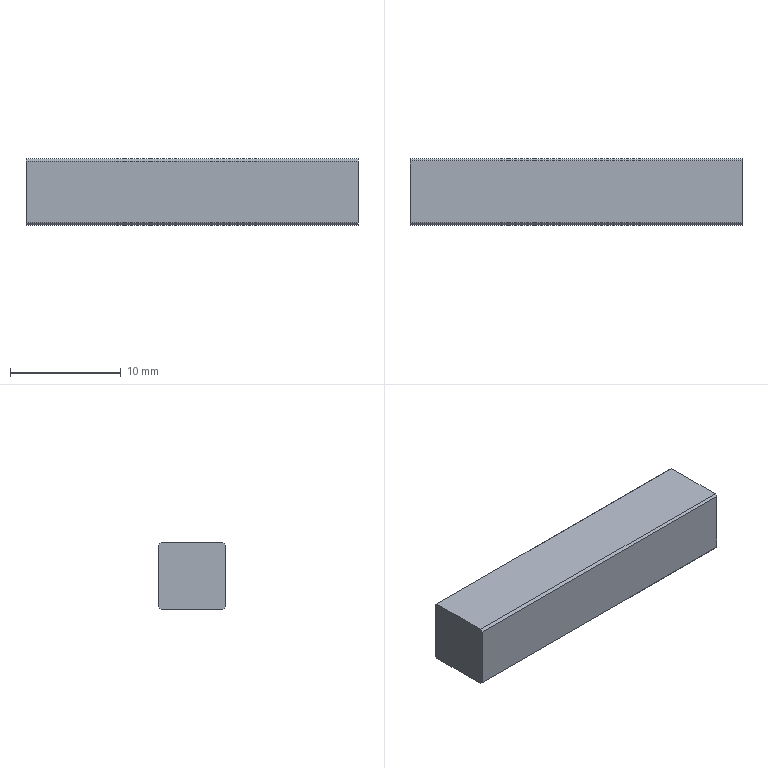Part | STEP file | KEDS6-30 | 1 solid | 10 faces | box 30 x 6 x 6 mm | volume 1078 mm3 | plane 10
STEP:
#1=CARTESIAN_POINT('',(-15.,6.,-2.8));
#2=VERTEX_POINT('',#1);
#3=CARTESIAN_POINT('',(-15.,6.,2.8));
#4=VERTEX_POINT('',#3);
#5=CARTESIAN_POINT('',(-15.,6.,-3.));
#6=DIRECTION('',(0.,0.,1.));
#7=VECTOR('',#6,1000.);
#8=LINE('',#5,#7);
#9=EDGE_CURVE('',#2,#4,#8,.T.);
#10=ORIENTED_EDGE('',*,*,#9,.F.);
#11=CARTESIAN_POINT('',(-15.,5.8,-3.));
#12=VERTEX_POINT('',#11);
#13=CARTESIAN_POINT('',(-15.,6.,-2.8));
#14=DIRECTION('',(0.,-0.7071,-0.7071));
#15=VECTOR('',#14,1000.);
#16=LINE('',#13,#15);
#17=EDGE_CURVE('',#2,#12,#16,.T.);
#18=ORIENTED_EDGE('',*,*,#17,.T.);
#19=CARTESIAN_POINT('',(-15.,0.2,-3.));
#20=VERTEX_POINT('',#19);
#21=CARTESIAN_POINT('',(-15.,6.,-3.));
#22=DIRECTION('',(0.,-1.,0.));
#23=VECTOR('',#22,1000.);
#24=LINE('',#21,#23);
#25=EDGE_CURVE('',#12,#20,#24,.T.);
#26=ORIENTED_EDGE('',*,*,#25,.T.);
#27=CARTESIAN_POINT('',(-15.,0.,-2.8));
#28=VERTEX_POINT('',#27);
#29=CARTESIAN_POINT('',(-15.,0.2,-3.));
#30=DIRECTION('',(0.,-0.7071,0.7071));
#31=VECTOR('',#30,1000.);
#32=LINE('',#29,#31);
#33=EDGE_CURVE('',#20,#28,#32,.T.);
#34=ORIENTED_EDGE('',*,*,#33,.T.);
#35=CARTESIAN_POINT('',(-15.,0.,2.8));
#36=VERTEX_POINT('',#35);
#37=CARTESIAN_POINT('',(-15.,0.,-3.));
#38=DIRECTION('',(0.,0.,1.));
#39=VECTOR('',#38,1000.);
#40=LINE('',#37,#39);
#41=EDGE_CURVE('',#28,#36,#40,.T.);
#42=ORIENTED_EDGE('',*,*,#41,.T.);
#43=CARTESIAN_POINT('',(-15.,0.2,3.));
#44=VERTEX_POINT('',#43);
#45=CARTESIAN_POINT('',(-15.,0.2,3.));
#46=DIRECTION('',(0.,0.7071,0.7071));
#47=VECTOR('',#46,1000.);
#48=LINE('',#45,#47);
#49=EDGE_CURVE('',#36,#44,#48,.T.);
#50=ORIENTED_EDGE('',*,*,#49,.T.);
#51=CARTESIAN_POINT('',(-15.,5.8,3.));
#52=VERTEX_POINT('',#51);
#53=CARTESIAN_POINT('',(-15.,6.,3.));
#54=DIRECTION('',(0.,-1.,0.));
#55=VECTOR('',#54,1000.);
#56=LINE('',#53,#55);
#57=EDGE_CURVE('',#52,#44,#56,.T.);
#58=ORIENTED_EDGE('',*,*,#57,.F.);
#59=CARTESIAN_POINT('',(-15.,6.,2.8));
#60=DIRECTION('',(0.,0.7071,-0.7071));
#61=VECTOR('',#60,1000.);
#62=LINE('',#59,#61);
#63=EDGE_CURVE('',#52,#4,#62,.T.);
#64=ORIENTED_EDGE('',*,*,#63,.T.);
#65=EDGE_LOOP('',(#10,#18,#26,#34,#42,#50,#58,#64));
#66=FACE_OUTER_BOUND('',#65,.T.);
#67=CARTESIAN_POINT('',(-15.,6.,-3.));
#68=DIRECTION('',(1.,0.,0.));
#69=DIRECTION('',(0.,0.,-1.));
#70=AXIS2_PLACEMENT_3D('',#67,#68,#69);
#71=PLANE('',#70);
#72=ADVANCED_FACE('',(#66),#71,.F.);
#73=ORIENTED_EDGE('',*,*,#57,.T.);
#74=CARTESIAN_POINT('',(15.,0.2,3.));
#75=VERTEX_POINT('',#74);
#76=CARTESIAN_POINT('',(-15.,0.2,3.));
#77=DIRECTION('',(1.,0.,0.));
#78=VECTOR('',#77,1000.);
#79=LINE('',#76,#78);
#80=EDGE_CURVE('',#44,#75,#79,.T.);
#81=ORIENTED_EDGE('',*,*,#80,.T.);
#82=CARTESIAN_POINT('',(15.,5.8,3.));
#83=VERTEX_POINT('',#82);
#84=CARTESIAN_POINT('',(15.,6.,3.));
#85=DIRECTION('',(0.,-1.,0.));
#86=VECTOR('',#85,1000.);
#87=LINE('',#84,#86);
#88=EDGE_CURVE('',#83,#75,#87,.T.);
#89=ORIENTED_EDGE('',*,*,#88,.F.);
#90=CARTESIAN_POINT('',(-15.,5.8,3.));
#91=DIRECTION('',(-1.,0.,0.));
#92=VECTOR('',#91,1000.);
#93=LINE('',#90,#92);
#94=EDGE_CURVE('',#83,#52,#93,.T.);
#95=ORIENTED_EDGE('',*,*,#94,.T.);
#96=EDGE_LOOP('',(#73,#81,#89,#95));
#97=FACE_OUTER_BOUND('',#96,.T.);
#98=CARTESIAN_POINT('',(-15.,6.,3.));
#99=DIRECTION('',(0.,0.,-1.));
#100=DIRECTION('',(-1.,0.,0.));
#101=AXIS2_PLACEMENT_3D('',#98,#99,#100);
#102=PLANE('',#101);
#103=ADVANCED_FACE('',(#97),#102,.F.);
#104=CARTESIAN_POINT('',(15.,5.8,-3.));
#105=VERTEX_POINT('',#104);
#106=CARTESIAN_POINT('',(15.,0.2,-3.));
#107=VERTEX_POINT('',#106);
#108=CARTESIAN_POINT('',(15.,6.,-3.));
#109=DIRECTION('',(0.,-1.,0.));
#110=VECTOR('',#109,1000.);
#111=LINE('',#108,#110);
#112=EDGE_CURVE('',#105,#107,#111,.T.);
#113=ORIENTED_EDGE('',*,*,#112,.F.);
#114=CARTESIAN_POINT('',(15.,6.,-2.8));
#115=VERTEX_POINT('',#114);
#116=CARTESIAN_POINT('',(15.,6.,-2.8));
#117=DIRECTION('',(0.,0.7071,0.7071));
#118=VECTOR('',#117,1000.);
#119=LINE('',#116,#118);
#120=EDGE_CURVE('',#105,#115,#119,.T.);
#121=ORIENTED_EDGE('',*,*,#120,.T.);
#122=CARTESIAN_POINT('',(15.,6.,2.8));
#123=VERTEX_POINT('',#122);
#124=CARTESIAN_POINT('',(15.,6.,-3.));
#125=DIRECTION('',(0.,0.,-1.));
#126=VECTOR('',#125,1000.);
#127=LINE('',#124,#126);
#128=EDGE_CURVE('',#123,#115,#127,.T.);
#129=ORIENTED_EDGE('',*,*,#128,.F.);
#130=CARTESIAN_POINT('',(15.,6.,2.8));
#131=DIRECTION('',(0.,-0.7071,0.7071));
#132=VECTOR('',#131,1000.);
#133=LINE('',#130,#132);
#134=EDGE_CURVE('',#123,#83,#133,.T.);
#135=ORIENTED_EDGE('',*,*,#134,.T.);
#136=ORIENTED_EDGE('',*,*,#88,.T.);
#137=CARTESIAN_POINT('',(15.,0.,2.8));
#138=VERTEX_POINT('',#137);
#139=CARTESIAN_POINT('',(15.,0.2,3.));
#140=DIRECTION('',(0.,-0.7071,-0.7071));
#141=VECTOR('',#140,1000.);
#142=LINE('',#139,#141);
#143=EDGE_CURVE('',#75,#138,#142,.T.);
#144=ORIENTED_EDGE('',*,*,#143,.T.);
#145=CARTESIAN_POINT('',(15.,0.,-2.8));
#146=VERTEX_POINT('',#145);
#147=CARTESIAN_POINT('',(15.,0.,-3.));
#148=DIRECTION('',(0.,0.,-1.));
#149=VECTOR('',#148,1000.);
#150=LINE('',#147,#149);
#151=EDGE_CURVE('',#138,#146,#150,.T.);
#152=ORIENTED_EDGE('',*,*,#151,.T.);
#153=CARTESIAN_POINT('',(15.,0.2,-3.));
#154=DIRECTION('',(0.,0.7071,-0.7071));
#155=VECTOR('',#154,1000.);
#156=LINE('',#153,#155);
#157=EDGE_CURVE('',#146,#107,#156,.T.);
#158=ORIENTED_EDGE('',*,*,#157,.T.);
#159=EDGE_LOOP('',(#113,#121,#129,#135,#136,#144,#152,#158));
#160=FACE_OUTER_BOUND('',#159,.T.);
#161=CARTESIAN_POINT('',(15.,6.,-3.));
#162=DIRECTION('',(-1.,0.,0.));
#163=DIRECTION('',(0.,0.,1.));
#164=AXIS2_PLACEMENT_3D('',#161,#162,#163);
#165=PLANE('',#164);
#166=ADVANCED_FACE('',(#160),#165,.F.);
#167=ORIENTED_EDGE('',*,*,#25,.F.);
#168=CARTESIAN_POINT('',(15.,5.8,-3.));
#169=DIRECTION('',(1.,0.,0.));
#170=VECTOR('',#169,1000.);
#171=LINE('',#168,#170);
#172=EDGE_CURVE('',#12,#105,#171,.T.);
#173=ORIENTED_EDGE('',*,*,#172,.T.);
#174=ORIENTED_EDGE('',*,*,#112,.T.);
#175=CARTESIAN_POINT('',(-15.,0.2,-3.));
#176=DIRECTION('',(-1.,0.,0.));
#177=VECTOR('',#176,1000.);
#178=LINE('',#175,#177);
#179=EDGE_CURVE('',#107,#20,#178,.T.);
#180=ORIENTED_EDGE('',*,*,#179,.T.);
#181=EDGE_LOOP('',(#167,#173,#174,#180));
#182=FACE_OUTER_BOUND('',#181,.T.);
#183=CARTESIAN_POINT('',(-15.,6.,-3.));
#184=DIRECTION('',(0.,0.,1.));
#185=DIRECTION('',(1.,0.,0.));
#186=AXIS2_PLACEMENT_3D('',#183,#184,#185);
#187=PLANE('',#186);
#188=ADVANCED_FACE('',(#182),#187,.F.);
#189=ORIENTED_EDGE('',*,*,#128,.T.);
#190=CARTESIAN_POINT('',(-15.,6.,-2.8));
#191=DIRECTION('',(-1.,0.,0.));
#192=VECTOR('',#191,1000.);
#193=LINE('',#190,#192);
#194=EDGE_CURVE('',#115,#2,#193,.T.);
#195=ORIENTED_EDGE('',*,*,#194,.T.);
#196=ORIENTED_EDGE('',*,*,#9,.T.);
#197=CARTESIAN_POINT('',(15.,6.,2.8));
#198=DIRECTION('',(1.,0.,0.));
#199=VECTOR('',#198,1000.);
#200=LINE('',#197,#199);
#201=EDGE_CURVE('',#4,#123,#200,.T.);
#202=ORIENTED_EDGE('',*,*,#201,.T.);
#203=EDGE_LOOP('',(#189,#195,#196,#202));
#204=FACE_OUTER_BOUND('',#203,.T.);
#205=CARTESIAN_POINT('',(0.,6.,0.));
#206=DIRECTION('',(0.,1.,0.));
#207=DIRECTION('',(0.,0.,1.));
#208=AXIS2_PLACEMENT_3D('',#205,#206,#207);
#209=PLANE('',#208);
#210=ADVANCED_FACE('',(#204),#209,.T.);
#211=ORIENTED_EDGE('',*,*,#41,.F.);
#212=CARTESIAN_POINT('',(0.,0.,-2.8));
#213=DIRECTION('',(1.,0.,0.));
#214=VECTOR('',#213,1000.);
#215=LINE('',#212,#214);
#216=EDGE_CURVE('',#28,#146,#215,.T.);
#217=ORIENTED_EDGE('',*,*,#216,.T.);
#218=ORIENTED_EDGE('',*,*,#151,.F.);
#219=CARTESIAN_POINT('',(0.,0.,2.8));
#220=DIRECTION('',(-1.,0.,0.));
#221=VECTOR('',#220,1000.);
#222=LINE('',#219,#221);
#223=EDGE_CURVE('',#138,#36,#222,.T.);
#224=ORIENTED_EDGE('',*,*,#223,.T.);
#225=EDGE_LOOP('',(#211,#217,#218,#224));
#226=FACE_OUTER_BOUND('',#225,.T.);
#227=CARTESIAN_POINT('',(0.,0.,0.));
#228=DIRECTION('',(0.,1.,0.));
#229=DIRECTION('',(0.,0.,1.));
#230=AXIS2_PLACEMENT_3D('',#227,#228,#229);
#231=PLANE('',#230);
#232=ADVANCED_FACE('',(#226),#231,.F.);
#233=ORIENTED_EDGE('',*,*,#120,.F.);
#234=ORIENTED_EDGE('',*,*,#172,.F.);
#235=ORIENTED_EDGE('',*,*,#17,.F.);
#236=ORIENTED_EDGE('',*,*,#194,.F.);
#237=EDGE_LOOP('',(#233,#234,#235,#236));
#238=FACE_OUTER_BOUND('',#237,.T.);
#239=CARTESIAN_POINT('',(0.,6.,-2.8));
#240=DIRECTION('',(0.,0.7071,-0.7071));
#241=DIRECTION('',(1.,0.,0.));
#242=AXIS2_PLACEMENT_3D('',#239,#240,#241);
#243=PLANE('',#242);
#244=ADVANCED_FACE('',(#238),#243,.T.);
#245=ORIENTED_EDGE('',*,*,#157,.F.);
#246=ORIENTED_EDGE('',*,*,#216,.F.);
#247=ORIENTED_EDGE('',*,*,#33,.F.);
#248=ORIENTED_EDGE('',*,*,#179,.F.);
#249=EDGE_LOOP('',(#245,#246,#247,#248));
#250=FACE_OUTER_BOUND('',#249,.T.);
#251=CARTESIAN_POINT('',(-15.,0.2,-3.));
#252=DIRECTION('',(0.,0.7071,0.7071));
#253=DIRECTION('',(-1.,0.,0.));
#254=AXIS2_PLACEMENT_3D('',#251,#252,#253);
#255=PLANE('',#254);
#256=ADVANCED_FACE('',(#250),#255,.F.);
#257=ORIENTED_EDGE('',*,*,#49,.F.);
#258=ORIENTED_EDGE('',*,*,#223,.F.);
#259=ORIENTED_EDGE('',*,*,#143,.F.);
#260=ORIENTED_EDGE('',*,*,#80,.F.);
#261=EDGE_LOOP('',(#257,#258,#259,#260));
#262=FACE_OUTER_BOUND('',#261,.T.);
#263=CARTESIAN_POINT('',(-15.,0.2,3.));
#264=DIRECTION('',(0.,0.7071,-0.7071));
#265=DIRECTION('',(1.,0.,0.));
#266=AXIS2_PLACEMENT_3D('',#263,#264,#265);
#267=PLANE('',#266);
#268=ADVANCED_FACE('',(#262),#267,.F.);
#269=ORIENTED_EDGE('',*,*,#63,.F.);
#270=ORIENTED_EDGE('',*,*,#94,.F.);
#271=ORIENTED_EDGE('',*,*,#134,.F.);
#272=ORIENTED_EDGE('',*,*,#201,.F.);
#273=EDGE_LOOP('',(#269,#270,#271,#272));
#274=FACE_OUTER_BOUND('',#273,.T.);
#275=CARTESIAN_POINT('',(0.,6.,2.8));
#276=DIRECTION('',(0.,0.7071,0.7071));
#277=DIRECTION('',(-1.,0.,0.));
#278=AXIS2_PLACEMENT_3D('',#275,#276,#277);
#279=PLANE('',#278);
#280=ADVANCED_FACE('',(#274),#279,.T.);
#281=CLOSED_SHELL('',(#72,#103,#166,#188,#210,#232,#244,#256,#268,#280));
#282=MANIFOLD_SOLID_BREP('',#281);
#283=CARTESIAN_POINT('',(0.,0.,0.));
#284=DIRECTION('',(0.,0.,1.));
#285=DIRECTION('',(1.,0.,0.));
#286=AXIS2_PLACEMENT_3D('',#283,#284,#285);
#287=(LENGTH_UNIT()NAMED_UNIT(*)SI_UNIT(.MILLI.,.METRE.));
#288=UNCERTAINTY_MEASURE_WITH_UNIT(LENGTH_MEASURE(0.00001),#287,'','');
#289=(NAMED_UNIT(*)PLANE_ANGLE_UNIT()SI_UNIT($,.RADIAN.));
#290=(NAMED_UNIT(*)SI_UNIT($,.STERADIAN.)SOLID_ANGLE_UNIT());
#291=(GEOMETRIC_REPRESENTATION_CONTEXT(3)GLOBAL_UNCERTAINTY_ASSIGNED_CONTEXT((#288))GLOBAL_UNIT_ASSIGNED_CONTEXT((#287,#289,#290))REPRESENTATION_CONTEXT('',''));
#292=ADVANCED_BREP_SHAPE_REPRESENTATION('',(#282,#286),#291);